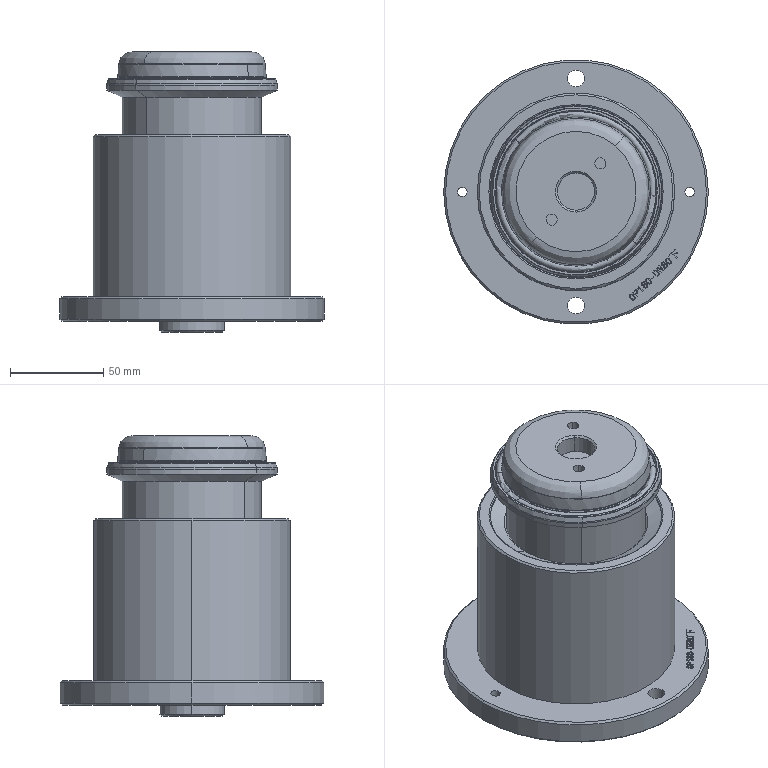Part | SolidWorks | 6 solids | 322 faces | box 142 x 142 x 150.5 mm | volume 760859 mm3 | plane 107 | spline 71 | cylinder 60 | cone 48 | torus 36 | commonest cylinder face diameters 5 x6 6 x6 8 x4 9 x4 17.5 x4 20 x4